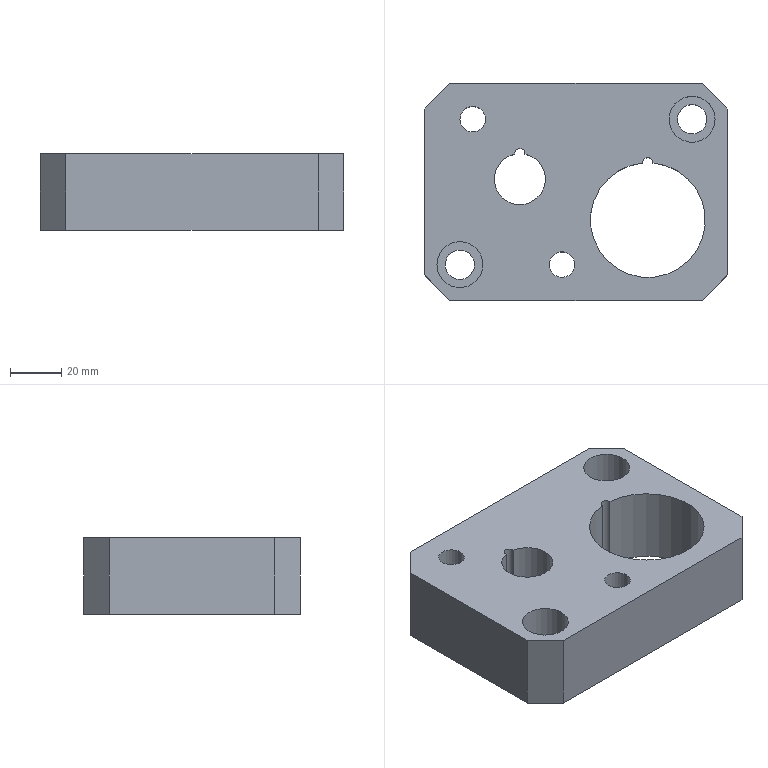Part | NX | features 23 2 | 1 solid | 22 faces | box 119 x 85 x 30 mm | volume 224460 mm3 | plane 12 | cylinder 10 | commonest cylinder face diameters 10.001 x2 11.5 x2 18 x2 4 x1 4.001 x1 20 x1
STEP:
#1=CARTESIAN_POINT('',(135.201,-405.589,-3.5));
#2=VERTEX_POINT('',#1);
#3=CARTESIAN_POINT('',(135.201,-405.589,-33.5));
#4=VERTEX_POINT('',#3);
#5=CARTESIAN_POINT('',(135.201,-405.589,66.5));
#6=DIRECTION('',(0.,0.,-1.));
#7=VECTOR('',#6,1000.);
#8=LINE('',#5,#7);
#9=EDGE_CURVE('',#2,#4,#8,.T.);
#10=ORIENTED_EDGE('',*,*,#9,.F.);
#11=CARTESIAN_POINT('',(139.198,-405.589,-3.5));
#12=VERTEX_POINT('',#11);
#13=CARTESIAN_POINT('',(137.199,-428.,-3.5));
#14=DIRECTION('',(0.,0.,1.));
#15=DIRECTION('',(-1.,0.,0.));
#16=AXIS2_PLACEMENT_3D('',#13,#14,#15);
#17=CIRCLE('',#16,22.5);
#18=EDGE_CURVE('',#2,#12,#17,.T.);
#19=ORIENTED_EDGE('',*,*,#18,.T.);
#20=CARTESIAN_POINT('',(139.198,-405.589,-33.5));
#21=VERTEX_POINT('',#20);
#22=CARTESIAN_POINT('',(139.198,-405.589,66.5));
#23=DIRECTION('',(0.,0.,1.));
#24=VECTOR('',#23,1000.);
#25=LINE('',#22,#24);
#26=EDGE_CURVE('',#21,#12,#25,.T.);
#27=ORIENTED_EDGE('',*,*,#26,.F.);
#28=CARTESIAN_POINT('',(137.199,-428.,-33.5));
#29=DIRECTION('',(0.,0.,-1.));
#30=DIRECTION('',(-1.,0.,0.));
#31=AXIS2_PLACEMENT_3D('',#28,#29,#30);
#32=CIRCLE('',#31,22.5);
#33=EDGE_CURVE('',#21,#4,#32,.T.);
#34=ORIENTED_EDGE('',*,*,#33,.T.);
#35=EDGE_LOOP('',(#10,#19,#27,#34));
#36=FACE_BOUND('',#35,.T.);
#37=CARTESIAN_POINT('',(137.199,-428.,-158.));
#38=DIRECTION('',(0.,0.,1.));
#39=DIRECTION('',(-1.,0.,0.));
#40=AXIS2_PLACEMENT_3D('',#37,#38,#39);
#41=CYLINDRICAL_SURFACE('',#40,22.5);
#42=ADVANCED_FACE('',(#36),#41,.F.);
#43=CARTESIAN_POINT('',(63.528,-388.45,-3.5));
#44=VERTEX_POINT('',#43);
#45=CARTESIAN_POINT('',(68.529,-388.45,-3.5));
#46=DIRECTION('',(0.,0.,-1.));
#47=DIRECTION('',(-1.,0.,0.));
#48=AXIS2_PLACEMENT_3D('',#45,#46,#47);
#49=CIRCLE('',#48,5.);
#50=EDGE_CURVE('',#44,#44,#49,.T.);
#51=ORIENTED_EDGE('',*,*,#50,.T.);
#52=EDGE_LOOP('',(#51));
#53=FACE_BOUND('',#52,.T.);
#54=CARTESIAN_POINT('',(145.529,-388.45,-3.5));
#55=VERTEX_POINT('',#54);
#56=CARTESIAN_POINT('',(154.529,-388.45,-3.5));
#57=DIRECTION('',(0.,0.,1.));
#58=DIRECTION('',(-1.,0.,0.));
#59=AXIS2_PLACEMENT_3D('',#56,#57,#58);
#60=CIRCLE('',#59,9.);
#61=EDGE_CURVE('',#55,#55,#60,.T.);
#62=ORIENTED_EDGE('',*,*,#61,.F.);
#63=EDGE_LOOP('',(#62));
#64=FACE_BOUND('',#63,.T.);
#65=CARTESIAN_POINT('',(158.529,-374.45,-3.5));
#66=VERTEX_POINT('',#65);
#67=CARTESIAN_POINT('',(59.529,-374.45,-3.5));
#68=VERTEX_POINT('',#67);
#69=CARTESIAN_POINT('',(87.029,-374.45,-3.5));
#70=DIRECTION('',(-1.,0.,0.));
#71=VECTOR('',#70,1000.);
#72=LINE('',#69,#71);
#73=EDGE_CURVE('',#66,#68,#72,.T.);
#74=ORIENTED_EDGE('',*,*,#73,.T.);
#75=CARTESIAN_POINT('',(49.529,-384.45,-3.5));
#76=VERTEX_POINT('',#75);
#77=CARTESIAN_POINT('',(37.227,-396.752,-3.5));
#78=DIRECTION('',(0.7071,0.7071,0.));
#79=VECTOR('',#78,1000.);
#80=LINE('',#77,#79);
#81=EDGE_CURVE('',#76,#68,#80,.T.);
#82=ORIENTED_EDGE('',*,*,#81,.F.);
#83=CARTESIAN_POINT('',(49.529,-449.45,-3.5));
#84=VERTEX_POINT('',#83);
#85=CARTESIAN_POINT('',(49.529,-411.95,-3.5));
#86=DIRECTION('',(0.,-1.,0.));
#87=VECTOR('',#86,1000.);
#88=LINE('',#85,#87);
#89=EDGE_CURVE('',#76,#84,#88,.T.);
#90=ORIENTED_EDGE('',*,*,#89,.T.);
#91=CARTESIAN_POINT('',(59.529,-459.45,-3.5));
#92=VERTEX_POINT('',#91);
#93=CARTESIAN_POINT('',(59.902,-459.824,-3.5));
#94=DIRECTION('',(-0.7071,0.7071,0.));
#95=VECTOR('',#94,1000.);
#96=LINE('',#93,#95);
#97=EDGE_CURVE('',#92,#84,#96,.T.);
#98=ORIENTED_EDGE('',*,*,#97,.F.);
#99=CARTESIAN_POINT('',(158.529,-459.45,-3.5));
#100=VERTEX_POINT('',#99);
#101=CARTESIAN_POINT('',(87.029,-459.45,-3.5));
#102=DIRECTION('',(1.,0.,0.));
#103=VECTOR('',#102,1000.);
#104=LINE('',#101,#103);
#105=EDGE_CURVE('',#92,#100,#104,.T.);
#106=ORIENTED_EDGE('',*,*,#105,.T.);
#107=CARTESIAN_POINT('',(168.529,-449.45,-3.5));
#108=VERTEX_POINT('',#107);
#109=CARTESIAN_POINT('',(151.227,-466.752,-3.5));
#110=DIRECTION('',(-0.7071,-0.7071,0.));
#111=VECTOR('',#110,1000.);
#112=LINE('',#109,#111);
#113=EDGE_CURVE('',#108,#100,#112,.T.);
#114=ORIENTED_EDGE('',*,*,#113,.F.);
#115=CARTESIAN_POINT('',(168.529,-384.45,-3.5));
#116=VERTEX_POINT('',#115);
#117=CARTESIAN_POINT('',(168.529,-411.95,-3.5));
#118=DIRECTION('',(0.,1.,0.));
#119=VECTOR('',#118,1000.);
#120=LINE('',#117,#119);
#121=EDGE_CURVE('',#108,#116,#120,.T.);
#122=ORIENTED_EDGE('',*,*,#121,.T.);
#123=CARTESIAN_POINT('',(173.902,-389.824,-3.5));
#124=DIRECTION('',(0.7071,-0.7071,0.));
#125=VECTOR('',#124,1000.);
#126=LINE('',#123,#125);
#127=EDGE_CURVE('',#66,#116,#126,.T.);
#128=ORIENTED_EDGE('',*,*,#127,.F.);
#129=EDGE_LOOP('',(#74,#82,#90,#98,#106,#114,#122,#128));
#130=FACE_BOUND('',#129,.T.);
#131=CARTESIAN_POINT('',(98.528,-445.45,-3.5));
#132=VERTEX_POINT('',#131);
#133=CARTESIAN_POINT('',(103.529,-445.45,-3.5));
#134=DIRECTION('',(0.,0.,-1.));
#135=DIRECTION('',(-1.,0.,0.));
#136=AXIS2_PLACEMENT_3D('',#133,#134,#135);
#137=CIRCLE('',#136,5.);
#138=EDGE_CURVE('',#132,#132,#137,.T.);
#139=ORIENTED_EDGE('',*,*,#138,.T.);
#140=EDGE_LOOP('',(#139));
#141=FACE_BOUND('',#140,.T.);
#142=CARTESIAN_POINT('',(54.529,-445.45,-3.5));
#143=VERTEX_POINT('',#142);
#144=CARTESIAN_POINT('',(63.529,-445.45,-3.5));
#145=DIRECTION('',(0.,0.,1.));
#146=DIRECTION('',(-1.,0.,0.));
#147=AXIS2_PLACEMENT_3D('',#144,#145,#146);
#148=CIRCLE('',#147,9.);
#149=EDGE_CURVE('',#143,#143,#148,.T.);
#150=ORIENTED_EDGE('',*,*,#149,.F.);
#151=EDGE_LOOP('',(#150));
#152=FACE_BOUND('',#151,.T.);
#153=CARTESIAN_POINT('',(89.019,-402.15,-3.5));
#154=VERTEX_POINT('',#153);
#155=CARTESIAN_POINT('',(85.039,-402.15,-3.5));
#156=VERTEX_POINT('',#155);
#157=CARTESIAN_POINT('',(87.029,-411.95,-3.5));
#158=DIRECTION('',(0.,0.,-1.));
#159=DIRECTION('',(-1.,0.,0.));
#160=AXIS2_PLACEMENT_3D('',#157,#158,#159);
#161=CIRCLE('',#160,10.);
#162=EDGE_CURVE('',#154,#156,#161,.T.);
#163=ORIENTED_EDGE('',*,*,#162,.T.);
#164=CARTESIAN_POINT('',(87.029,-401.95,-3.5));
#165=DIRECTION('',(0.,0.,-1.));
#166=DIRECTION('',(-1.,0.,0.));
#167=AXIS2_PLACEMENT_3D('',#164,#165,#166);
#168=CIRCLE('',#167,2.);
#169=EDGE_CURVE('',#156,#154,#168,.T.);
#170=ORIENTED_EDGE('',*,*,#169,.T.);
#171=EDGE_LOOP('',(#163,#170));
#172=FACE_BOUND('',#171,.T.);
#173=ORIENTED_EDGE('',*,*,#18,.F.);
#174=CARTESIAN_POINT('',(137.199,-405.5,-3.5));
#175=DIRECTION('',(0.,0.,-1.));
#176=DIRECTION('',(-1.,0.,0.));
#177=AXIS2_PLACEMENT_3D('',#174,#175,#176);
#178=CIRCLE('',#177,2.001);
#179=EDGE_CURVE('',#2,#12,#178,.T.);
#180=ORIENTED_EDGE('',*,*,#179,.T.);
#181=EDGE_LOOP('',(#173,#180));
#182=FACE_BOUND('',#181,.T.);
#183=CARTESIAN_POINT('',(80.101,-434.625,-3.5));
#184=DIRECTION('',(0.,0.,-1.));
#185=DIRECTION('',(-1.,0.,0.));
#186=AXIS2_PLACEMENT_3D('',#183,#184,#185);
#187=PLANE('',#186);
#188=ADVANCED_FACE('',(#53,#64,#130,#141,#152,#172,#182),#187,.F.);
#189=CARTESIAN_POINT('',(137.199,-405.5,-33.5));
#190=DIRECTION('',(0.,0.,1.));
#191=DIRECTION('',(1.,0.,0.));
#192=AXIS2_PLACEMENT_3D('',#189,#190,#191);
#193=CIRCLE('',#192,2.001);
#194=EDGE_CURVE('',#21,#4,#193,.T.);
#195=ORIENTED_EDGE('',*,*,#194,.T.);
#196=ORIENTED_EDGE('',*,*,#33,.F.);
#197=EDGE_LOOP('',(#195,#196));
#198=FACE_BOUND('',#197,.T.);
#199=CARTESIAN_POINT('',(168.529,-384.45,-33.5));
#200=VERTEX_POINT('',#199);
#201=CARTESIAN_POINT('',(168.529,-449.45,-33.5));
#202=VERTEX_POINT('',#201);
#203=CARTESIAN_POINT('',(168.529,-411.95,-33.5));
#204=DIRECTION('',(0.,-1.,0.));
#205=VECTOR('',#204,1000.);
#206=LINE('',#203,#205);
#207=EDGE_CURVE('',#200,#202,#206,.T.);
#208=ORIENTED_EDGE('',*,*,#207,.T.);
#209=CARTESIAN_POINT('',(158.529,-459.45,-33.5));
#210=VERTEX_POINT('',#209);
#211=CARTESIAN_POINT('',(199.464,-418.515,-33.5));
#212=DIRECTION('',(0.7071,0.7071,0.));
#213=VECTOR('',#212,1000.);
#214=LINE('',#211,#213);
#215=EDGE_CURVE('',#210,#202,#214,.T.);
#216=ORIENTED_EDGE('',*,*,#215,.F.);
#217=CARTESIAN_POINT('',(59.529,-459.45,-33.5));
#218=VERTEX_POINT('',#217);
#219=CARTESIAN_POINT('',(87.029,-459.45,-33.5));
#220=DIRECTION('',(-1.,0.,0.));
#221=VECTOR('',#220,1000.);
#222=LINE('',#219,#221);
#223=EDGE_CURVE('',#210,#218,#222,.T.);
#224=ORIENTED_EDGE('',*,*,#223,.T.);
#225=CARTESIAN_POINT('',(49.529,-449.45,-33.5));
#226=VERTEX_POINT('',#225);
#227=CARTESIAN_POINT('',(51.02,-450.941,-33.5));
#228=DIRECTION('',(0.7071,-0.7071,0.));
#229=VECTOR('',#228,1000.);
#230=LINE('',#227,#229);
#231=EDGE_CURVE('',#226,#218,#230,.T.);
#232=ORIENTED_EDGE('',*,*,#231,.F.);
#233=CARTESIAN_POINT('',(49.529,-384.45,-33.5));
#234=VERTEX_POINT('',#233);
#235=CARTESIAN_POINT('',(49.529,-411.95,-33.5));
#236=DIRECTION('',(0.,1.,0.));
#237=VECTOR('',#236,1000.);
#238=LINE('',#235,#237);
#239=EDGE_CURVE('',#226,#234,#238,.T.);
#240=ORIENTED_EDGE('',*,*,#239,.T.);
#241=CARTESIAN_POINT('',(59.529,-374.45,-33.5));
#242=VERTEX_POINT('',#241);
#243=CARTESIAN_POINT('',(85.464,-348.515,-33.5));
#244=DIRECTION('',(-0.7071,-0.7071,0.));
#245=VECTOR('',#244,1000.);
#246=LINE('',#243,#245);
#247=EDGE_CURVE('',#242,#234,#246,.T.);
#248=ORIENTED_EDGE('',*,*,#247,.F.);
#249=CARTESIAN_POINT('',(158.529,-374.45,-33.5));
#250=VERTEX_POINT('',#249);
#251=CARTESIAN_POINT('',(87.029,-374.45,-33.5));
#252=DIRECTION('',(1.,0.,0.));
#253=VECTOR('',#252,1000.);
#254=LINE('',#251,#253);
#255=EDGE_CURVE('',#242,#250,#254,.T.);
#256=ORIENTED_EDGE('',*,*,#255,.T.);
#257=CARTESIAN_POINT('',(165.02,-380.941,-33.5));
#258=DIRECTION('',(-0.7071,0.7071,0.));
#259=VECTOR('',#258,1000.);
#260=LINE('',#257,#259);
#261=EDGE_CURVE('',#200,#250,#260,.T.);
#262=ORIENTED_EDGE('',*,*,#261,.F.);
#263=EDGE_LOOP('',(#208,#216,#224,#232,#240,#248,#256,#262));
#264=FACE_BOUND('',#263,.T.);
#265=CARTESIAN_POINT('',(148.779,-388.45,-33.5));
#266=VERTEX_POINT('',#265);
#267=CARTESIAN_POINT('',(154.529,-388.45,-33.5));
#268=DIRECTION('',(0.,0.,1.));
#269=DIRECTION('',(-1.,0.,0.));
#270=AXIS2_PLACEMENT_3D('',#267,#268,#269);
#271=CIRCLE('',#270,5.75);
#272=EDGE_CURVE('',#266,#266,#271,.T.);
#273=ORIENTED_EDGE('',*,*,#272,.T.);
#274=EDGE_LOOP('',(#273));
#275=FACE_BOUND('',#274,.T.);
#276=CARTESIAN_POINT('',(98.528,-445.45,-33.5));
#277=VERTEX_POINT('',#276);
#278=CARTESIAN_POINT('',(103.529,-445.45,-33.5));
#279=DIRECTION('',(0.,0.,1.));
#280=DIRECTION('',(-1.,0.,0.));
#281=AXIS2_PLACEMENT_3D('',#278,#279,#280);
#282=CIRCLE('',#281,5.);
#283=EDGE_CURVE('',#277,#277,#282,.T.);
#284=ORIENTED_EDGE('',*,*,#283,.T.);
#285=EDGE_LOOP('',(#284));
#286=FACE_BOUND('',#285,.T.);
#287=CARTESIAN_POINT('',(57.779,-445.45,-33.5));
#288=VERTEX_POINT('',#287);
#289=CARTESIAN_POINT('',(63.529,-445.45,-33.5));
#290=DIRECTION('',(0.,0.,1.));
#291=DIRECTION('',(-1.,0.,0.));
#292=AXIS2_PLACEMENT_3D('',#289,#290,#291);
#293=CIRCLE('',#292,5.75);
#294=EDGE_CURVE('',#288,#288,#293,.T.);
#295=ORIENTED_EDGE('',*,*,#294,.T.);
#296=EDGE_LOOP('',(#295));
#297=FACE_BOUND('',#296,.T.);
#298=CARTESIAN_POINT('',(63.528,-388.45,-33.5));
#299=VERTEX_POINT('',#298);
#300=CARTESIAN_POINT('',(68.529,-388.45,-33.5));
#301=DIRECTION('',(0.,0.,1.));
#302=DIRECTION('',(-1.,0.,0.));
#303=AXIS2_PLACEMENT_3D('',#300,#301,#302);
#304=CIRCLE('',#303,5.);
#305=EDGE_CURVE('',#299,#299,#304,.T.);
#306=ORIENTED_EDGE('',*,*,#305,.T.);
#307=EDGE_LOOP('',(#306));
#308=FACE_BOUND('',#307,.T.);
#309=CARTESIAN_POINT('',(89.019,-402.15,-33.5));
#310=VERTEX_POINT('',#309);
#311=CARTESIAN_POINT('',(85.039,-402.15,-33.5));
#312=VERTEX_POINT('',#311);
#313=CARTESIAN_POINT('',(87.029,-401.95,-33.5));
#314=DIRECTION('',(0.,0.,1.));
#315=DIRECTION('',(1.,0.,0.));
#316=AXIS2_PLACEMENT_3D('',#313,#314,#315);
#317=CIRCLE('',#316,2.);
#318=EDGE_CURVE('',#310,#312,#317,.T.);
#319=ORIENTED_EDGE('',*,*,#318,.T.);
#320=CARTESIAN_POINT('',(87.029,-411.95,-33.5));
#321=DIRECTION('',(0.,0.,1.));
#322=DIRECTION('',(-1.,0.,0.));
#323=AXIS2_PLACEMENT_3D('',#320,#321,#322);
#324=CIRCLE('',#323,10.);
#325=EDGE_CURVE('',#312,#310,#324,.T.);
#326=ORIENTED_EDGE('',*,*,#325,.T.);
#327=EDGE_LOOP('',(#319,#326));
#328=FACE_BOUND('',#327,.T.);
#329=CARTESIAN_POINT('',(119.455,-377.506,-33.5));
#330=DIRECTION('',(0.,0.,-1.));
#331=DIRECTION('',(-1.,0.,0.));
#332=AXIS2_PLACEMENT_3D('',#329,#330,#331);
#333=PLANE('',#332);
#334=ADVANCED_FACE('',(#198,#264,#275,#286,#297,#308,#328),#333,.T.);
#335=CARTESIAN_POINT('',(148.779,-388.45,-18.5));
#336=VERTEX_POINT('',#335);
#337=CARTESIAN_POINT('',(154.529,-388.45,-18.5));
#338=DIRECTION('',(0.,0.,1.));
#339=DIRECTION('',(-1.,0.,0.));
#340=AXIS2_PLACEMENT_3D('',#337,#338,#339);
#341=CIRCLE('',#340,5.75);
#342=EDGE_CURVE('',#336,#336,#341,.T.);
#343=ORIENTED_EDGE('',*,*,#342,.F.);
#344=EDGE_LOOP('',(#343));
#345=FACE_BOUND('',#344,.T.);
#346=CARTESIAN_POINT('',(145.529,-388.45,-18.5));
#347=VERTEX_POINT('',#346);
#348=CARTESIAN_POINT('',(154.529,-388.45,-18.5));
#349=DIRECTION('',(0.,0.,1.));
#350=DIRECTION('',(-1.,0.,0.));
#351=AXIS2_PLACEMENT_3D('',#348,#349,#350);
#352=CIRCLE('',#351,9.);
#353=EDGE_CURVE('',#347,#347,#352,.T.);
#354=ORIENTED_EDGE('',*,*,#353,.T.);
#355=EDGE_LOOP('',(#354));
#356=FACE_BOUND('',#355,.T.);
#357=CARTESIAN_POINT('',(154.529,-388.45,-18.5));
#358=DIRECTION('',(0.,0.,-1.));
#359=DIRECTION('',(-1.,0.,0.));
#360=AXIS2_PLACEMENT_3D('',#357,#358,#359);
#361=PLANE('',#360);
#362=ADVANCED_FACE('',(#345,#356),#361,.F.);
#363=CARTESIAN_POINT('',(57.779,-445.45,-18.5));
#364=VERTEX_POINT('',#363);
#365=CARTESIAN_POINT('',(63.529,-445.45,-18.5));
#366=DIRECTION('',(0.,0.,1.));
#367=DIRECTION('',(-1.,0.,0.));
#368=AXIS2_PLACEMENT_3D('',#365,#366,#367);
#369=CIRCLE('',#368,5.75);
#370=EDGE_CURVE('',#364,#364,#369,.T.);
#371=ORIENTED_EDGE('',*,*,#370,.F.);
#372=EDGE_LOOP('',(#371));
#373=FACE_BOUND('',#372,.T.);
#374=CARTESIAN_POINT('',(54.529,-445.45,-18.5));
#375=VERTEX_POINT('',#374);
#376=CARTESIAN_POINT('',(63.529,-445.45,-18.5));
#377=DIRECTION('',(0.,0.,1.));
#378=DIRECTION('',(-1.,0.,0.));
#379=AXIS2_PLACEMENT_3D('',#376,#377,#378);
#380=CIRCLE('',#379,9.);
#381=EDGE_CURVE('',#375,#375,#380,.T.);
#382=ORIENTED_EDGE('',*,*,#381,.T.);
#383=EDGE_LOOP('',(#382));
#384=FACE_BOUND('',#383,.T.);
#385=CARTESIAN_POINT('',(63.529,-440.45,-18.5));
#386=DIRECTION('',(0.,0.,-1.));
#387=DIRECTION('',(-1.,0.,0.));
#388=AXIS2_PLACEMENT_3D('',#385,#386,#387);
#389=PLANE('',#388);
#390=ADVANCED_FACE('',(#373,#384),#389,.F.);
#391=ORIENTED_EDGE('',*,*,#272,.F.);
#392=EDGE_LOOP('',(#391));
#393=FACE_BOUND('',#392,.T.);
#394=ORIENTED_EDGE('',*,*,#342,.T.);
#395=EDGE_LOOP('',(#394));
#396=FACE_BOUND('',#395,.T.);
#397=CARTESIAN_POINT('',(154.529,-388.45,-1.5));
#398=DIRECTION('',(0.,0.,-1.));
#399=DIRECTION('',(1.,0.,0.));
#400=AXIS2_PLACEMENT_3D('',#397,#398,#399);
#401=CYLINDRICAL_SURFACE('',#400,5.75);
#402=ADVANCED_FACE('',(#393,#396),#401,.F.);
#403=ORIENTED_EDGE('',*,*,#294,.F.);
#404=EDGE_LOOP('',(#403));
#405=FACE_BOUND('',#404,.T.);
#406=ORIENTED_EDGE('',*,*,#370,.T.);
#407=EDGE_LOOP('',(#406));
#408=FACE_BOUND('',#407,.T.);
#409=CARTESIAN_POINT('',(63.529,-445.45,-1.5));
#410=DIRECTION('',(0.,0.,-1.));
#411=DIRECTION('',(1.,0.,0.));
#412=AXIS2_PLACEMENT_3D('',#409,#410,#411);
#413=CYLINDRICAL_SURFACE('',#412,5.75);
#414=ADVANCED_FACE('',(#405,#408),#413,.F.);
#415=ORIENTED_EDGE('',*,*,#50,.F.);
#416=EDGE_LOOP('',(#415));
#417=FACE_BOUND('',#416,.T.);
#418=ORIENTED_EDGE('',*,*,#305,.F.);
#419=EDGE_LOOP('',(#418));
#420=FACE_BOUND('',#419,.T.);
#421=CARTESIAN_POINT('',(68.529,-388.45,198.5));
#422=DIRECTION('',(0.,0.,-1.));
#423=DIRECTION('',(-1.,0.,0.));
#424=AXIS2_PLACEMENT_3D('',#421,#422,#423);
#425=CYLINDRICAL_SURFACE('',#424,5.);
#426=ADVANCED_FACE('',(#417,#420),#425,.F.);
#427=ORIENTED_EDGE('',*,*,#353,.F.);
#428=EDGE_LOOP('',(#427));
#429=FACE_BOUND('',#428,.T.);
#430=ORIENTED_EDGE('',*,*,#61,.T.);
#431=EDGE_LOOP('',(#430));
#432=FACE_BOUND('',#431,.T.);
#433=CARTESIAN_POINT('',(154.529,-388.45,-3.5));
#434=DIRECTION('',(0.,0.,-1.));
#435=DIRECTION('',(1.,0.,0.));
#436=AXIS2_PLACEMENT_3D('',#433,#434,#435);
#437=CYLINDRICAL_SURFACE('',#436,9.);
#438=ADVANCED_FACE('',(#429,#432),#437,.F.);
#439=ORIENTED_EDGE('',*,*,#261,.T.);
#440=CARTESIAN_POINT('',(158.529,-374.45,-23.5));
#441=DIRECTION('',(0.,0.,1.));
#442=VECTOR('',#441,1000.);
#443=LINE('',#440,#442);
#444=EDGE_CURVE('',#250,#66,#443,.T.);
#445=ORIENTED_EDGE('',*,*,#444,.T.);
#446=ORIENTED_EDGE('',*,*,#127,.T.);
#447=CARTESIAN_POINT('',(168.529,-384.45,-23.5));
#448=DIRECTION('',(0.,0.,-1.));
#449=VECTOR('',#448,1000.);
#450=LINE('',#447,#449);
#451=EDGE_CURVE('',#116,#200,#450,.T.);
#452=ORIENTED_EDGE('',*,*,#451,.T.);
#453=EDGE_LOOP('',(#439,#445,#446,#452));
#454=FACE_BOUND('',#453,.T.);
#455=CARTESIAN_POINT('',(163.529,-379.45,-23.5));
#456=DIRECTION('',(-0.7071,-0.7071,0.));
#457=DIRECTION('',(0.,0.,1.));
#458=AXIS2_PLACEMENT_3D('',#455,#456,#457);
#459=PLANE('',#458);
#460=ADVANCED_FACE('',(#454),#459,.F.);
#461=ORIENTED_EDGE('',*,*,#121,.F.);
#462=CARTESIAN_POINT('',(168.529,-449.45,-23.5));
#463=DIRECTION('',(0.,0.,1.));
#464=VECTOR('',#463,1000.);
#465=LINE('',#462,#464);
#466=EDGE_CURVE('',#202,#108,#465,.T.);
#467=ORIENTED_EDGE('',*,*,#466,.F.);
#468=ORIENTED_EDGE('',*,*,#207,.F.);
#469=ORIENTED_EDGE('',*,*,#451,.F.);
#470=EDGE_LOOP('',(#461,#467,#468,#469));
#471=FACE_BOUND('',#470,.T.);
#472=CARTESIAN_POINT('',(168.529,-411.95,-23.5));
#473=DIRECTION('',(1.,0.,0.));
#474=DIRECTION('',(0.,0.,-1.));
#475=AXIS2_PLACEMENT_3D('',#472,#473,#474);
#476=PLANE('',#475);
#477=ADVANCED_FACE('',(#471),#476,.T.);
#478=ORIENTED_EDGE('',*,*,#215,.T.);
#479=ORIENTED_EDGE('',*,*,#466,.T.);
#480=ORIENTED_EDGE('',*,*,#113,.T.);
#481=CARTESIAN_POINT('',(158.529,-459.45,-23.5));
#482=DIRECTION('',(0.,0.,-1.));
#483=VECTOR('',#482,1000.);
#484=LINE('',#481,#483);
#485=EDGE_CURVE('',#100,#210,#484,.T.);
#486=ORIENTED_EDGE('',*,*,#485,.T.);
#487=EDGE_LOOP('',(#478,#479,#480,#486));
#488=FACE_BOUND('',#487,.T.);
#489=CARTESIAN_POINT('',(168.529,-449.45,-23.5));
#490=DIRECTION('',(-0.7071,0.7071,0.));
#491=DIRECTION('',(0.,0.,1.));
#492=AXIS2_PLACEMENT_3D('',#489,#490,#491);
#493=PLANE('',#492);
#494=ADVANCED_FACE('',(#488),#493,.F.);
#495=ORIENTED_EDGE('',*,*,#105,.F.);
#496=CARTESIAN_POINT('',(59.529,-459.45,-23.5));
#497=DIRECTION('',(0.,0.,1.));
#498=VECTOR('',#497,1000.);
#499=LINE('',#496,#498);
#500=EDGE_CURVE('',#218,#92,#499,.T.);
#501=ORIENTED_EDGE('',*,*,#500,.F.);
#502=ORIENTED_EDGE('',*,*,#223,.F.);
#503=ORIENTED_EDGE('',*,*,#485,.F.);
#504=EDGE_LOOP('',(#495,#501,#502,#503));
#505=FACE_BOUND('',#504,.T.);
#506=CARTESIAN_POINT('',(87.029,-459.45,-23.5));
#507=DIRECTION('',(0.,-1.,0.));
#508=DIRECTION('',(0.,0.,1.));
#509=AXIS2_PLACEMENT_3D('',#506,#507,#508);
#510=PLANE('',#509);
#511=ADVANCED_FACE('',(#505),#510,.T.);
#512=ORIENTED_EDGE('',*,*,#231,.T.);
#513=ORIENTED_EDGE('',*,*,#500,.T.);
#514=ORIENTED_EDGE('',*,*,#97,.T.);
#515=CARTESIAN_POINT('',(49.529,-449.45,-23.5));
#516=DIRECTION('',(0.,0.,-1.));
#517=VECTOR('',#516,1000.);
#518=LINE('',#515,#517);
#519=EDGE_CURVE('',#84,#226,#518,.T.);
#520=ORIENTED_EDGE('',*,*,#519,.T.);
#521=EDGE_LOOP('',(#512,#513,#514,#520));
#522=FACE_BOUND('',#521,.T.);
#523=CARTESIAN_POINT('',(54.529,-454.45,-23.5));
#524=DIRECTION('',(0.7071,0.7071,0.));
#525=DIRECTION('',(0.,0.,1.));
#526=AXIS2_PLACEMENT_3D('',#523,#524,#525);
#527=PLANE('',#526);
#528=ADVANCED_FACE('',(#522),#527,.F.);
#529=ORIENTED_EDGE('',*,*,#89,.F.);
#530=CARTESIAN_POINT('',(49.529,-384.45,-23.5));
#531=DIRECTION('',(0.,0.,1.));
#532=VECTOR('',#531,1000.);
#533=LINE('',#530,#532);
#534=EDGE_CURVE('',#234,#76,#533,.T.);
#535=ORIENTED_EDGE('',*,*,#534,.F.);
#536=ORIENTED_EDGE('',*,*,#239,.F.);
#537=ORIENTED_EDGE('',*,*,#519,.F.);
#538=EDGE_LOOP('',(#529,#535,#536,#537));
#539=FACE_BOUND('',#538,.T.);
#540=CARTESIAN_POINT('',(49.529,-411.95,-23.5));
#541=DIRECTION('',(-1.,0.,0.));
#542=DIRECTION('',(0.,0.,1.));
#543=AXIS2_PLACEMENT_3D('',#540,#541,#542);
#544=PLANE('',#543);
#545=ADVANCED_FACE('',(#539),#544,.T.);
#546=ORIENTED_EDGE('',*,*,#247,.T.);
#547=ORIENTED_EDGE('',*,*,#534,.T.);
#548=ORIENTED_EDGE('',*,*,#81,.T.);
#549=CARTESIAN_POINT('',(59.529,-374.45,-23.5));
#550=DIRECTION('',(0.,0.,-1.));
#551=VECTOR('',#550,1000.);
#552=LINE('',#549,#551);
#553=EDGE_CURVE('',#68,#242,#552,.T.);
#554=ORIENTED_EDGE('',*,*,#553,.T.);
#555=EDGE_LOOP('',(#546,#547,#548,#554));
#556=FACE_BOUND('',#555,.T.);
#557=CARTESIAN_POINT('',(49.529,-384.45,-23.5));
#558=DIRECTION('',(0.7071,-0.7071,0.));
#559=DIRECTION('',(0.,0.,1.));
#560=AXIS2_PLACEMENT_3D('',#557,#558,#559);
#561=PLANE('',#560);
#562=ADVANCED_FACE('',(#556),#561,.F.);
#563=ORIENTED_EDGE('',*,*,#255,.F.);
#564=ORIENTED_EDGE('',*,*,#553,.F.);
#565=ORIENTED_EDGE('',*,*,#73,.F.);
#566=ORIENTED_EDGE('',*,*,#444,.F.);
#567=EDGE_LOOP('',(#563,#564,#565,#566));
#568=FACE_BOUND('',#567,.T.);
#569=CARTESIAN_POINT('',(87.029,-374.45,-23.5));
#570=DIRECTION('',(0.,1.,0.));
#571=DIRECTION('',(0.,0.,-1.));
#572=AXIS2_PLACEMENT_3D('',#569,#570,#571);
#573=PLANE('',#572);
#574=ADVANCED_FACE('',(#568),#573,.T.);
#575=ORIENTED_EDGE('',*,*,#138,.F.);
#576=EDGE_LOOP('',(#575));
#577=FACE_BOUND('',#576,.T.);
#578=ORIENTED_EDGE('',*,*,#283,.F.);
#579=EDGE_LOOP('',(#578));
#580=FACE_BOUND('',#579,.T.);
#581=CARTESIAN_POINT('',(103.529,-445.45,198.5));
#582=DIRECTION('',(0.,0.,-1.));
#583=DIRECTION('',(-1.,0.,0.));
#584=AXIS2_PLACEMENT_3D('',#581,#582,#583);
#585=CYLINDRICAL_SURFACE('',#584,5.);
#586=ADVANCED_FACE('',(#577,#580),#585,.F.);
#587=ORIENTED_EDGE('',*,*,#381,.F.);
#588=EDGE_LOOP('',(#587));
#589=FACE_BOUND('',#588,.T.);
#590=ORIENTED_EDGE('',*,*,#149,.T.);
#591=EDGE_LOOP('',(#590));
#592=FACE_BOUND('',#591,.T.);
#593=CARTESIAN_POINT('',(63.529,-445.45,-3.5));
#594=DIRECTION('',(0.,0.,-1.));
#595=DIRECTION('',(1.,0.,0.));
#596=AXIS2_PLACEMENT_3D('',#593,#594,#595);
#597=CYLINDRICAL_SURFACE('',#596,9.);
#598=ADVANCED_FACE('',(#589,#592),#597,.F.);
#599=ORIENTED_EDGE('',*,*,#325,.F.);
#600=CARTESIAN_POINT('',(85.039,-402.15,16.5));
#601=DIRECTION('',(0.,0.,1.));
#602=VECTOR('',#601,1000.);
#603=LINE('',#600,#602);
#604=EDGE_CURVE('',#312,#156,#603,.T.);
#605=ORIENTED_EDGE('',*,*,#604,.T.);
#606=ORIENTED_EDGE('',*,*,#162,.F.);
#607=CARTESIAN_POINT('',(89.019,-402.15,16.5));
#608=DIRECTION('',(0.,0.,-1.));
#609=VECTOR('',#608,1000.);
#610=LINE('',#607,#609);
#611=EDGE_CURVE('',#154,#310,#610,.T.);
#612=ORIENTED_EDGE('',*,*,#611,.T.);
#613=EDGE_LOOP('',(#599,#605,#606,#612));
#614=FACE_BOUND('',#613,.T.);
#615=CARTESIAN_POINT('',(87.029,-411.95,-18.5));
#616=DIRECTION('',(0.,0.,1.));
#617=DIRECTION('',(1.,0.,0.));
#618=AXIS2_PLACEMENT_3D('',#615,#616,#617);
#619=CYLINDRICAL_SURFACE('',#618,10.);
#620=ADVANCED_FACE('',(#614),#619,.F.);
#621=ORIENTED_EDGE('',*,*,#318,.F.);
#622=ORIENTED_EDGE('',*,*,#611,.F.);
#623=ORIENTED_EDGE('',*,*,#169,.F.);
#624=ORIENTED_EDGE('',*,*,#604,.F.);
#625=EDGE_LOOP('',(#621,#622,#623,#624));
#626=FACE_BOUND('',#625,.T.);
#627=CARTESIAN_POINT('',(87.029,-401.95,-33.5));
#628=DIRECTION('',(0.,0.,1.));
#629=DIRECTION('',(-1.,0.,0.));
#630=AXIS2_PLACEMENT_3D('',#627,#628,#629);
#631=CYLINDRICAL_SURFACE('',#630,2.);
#632=ADVANCED_FACE('',(#626),#631,.F.);
#633=ORIENTED_EDGE('',*,*,#9,.T.);
#634=ORIENTED_EDGE('',*,*,#194,.F.);
#635=ORIENTED_EDGE('',*,*,#26,.T.);
#636=ORIENTED_EDGE('',*,*,#179,.F.);
#637=EDGE_LOOP('',(#633,#634,#635,#636));
#638=FACE_BOUND('',#637,.T.);
#639=CARTESIAN_POINT('',(137.199,-405.5,-33.5));
#640=DIRECTION('',(0.,0.,1.));
#641=DIRECTION('',(-1.,0.,0.));
#642=AXIS2_PLACEMENT_3D('',#639,#640,#641);
#643=CYLINDRICAL_SURFACE('',#642,2.001);
#644=ADVANCED_FACE('',(#638),#643,.F.);
#645=CLOSED_SHELL('',(#42,#188,#334,#362,#390,#402,#414,#426,#438,#460,#477,#494,#511,#528,#545,#562,#574,#586,#598,#620,#632,#644));
#646=MANIFOLD_SOLID_BREP('',#645);
#647=(LENGTH_UNIT()NAMED_UNIT(*)SI_UNIT(.MILLI.,.METRE.));
#648=UNCERTAINTY_MEASURE_WITH_UNIT(LENGTH_MEASURE(0.00001),#647,'','');
#649=(NAMED_UNIT(*)PLANE_ANGLE_UNIT()SI_UNIT($,.RADIAN.));
#650=(NAMED_UNIT(*)SI_UNIT($,.STERADIAN.)SOLID_ANGLE_UNIT());
#651=(GEOMETRIC_REPRESENTATION_CONTEXT(3)GLOBAL_UNCERTAINTY_ASSIGNED_CONTEXT((#648))GLOBAL_UNIT_ASSIGNED_CONTEXT((#647,#649,#650))REPRESENTATION_CONTEXT('',''));
#652=ADVANCED_BREP_SHAPE_REPRESENTATION('',(#646),#651);